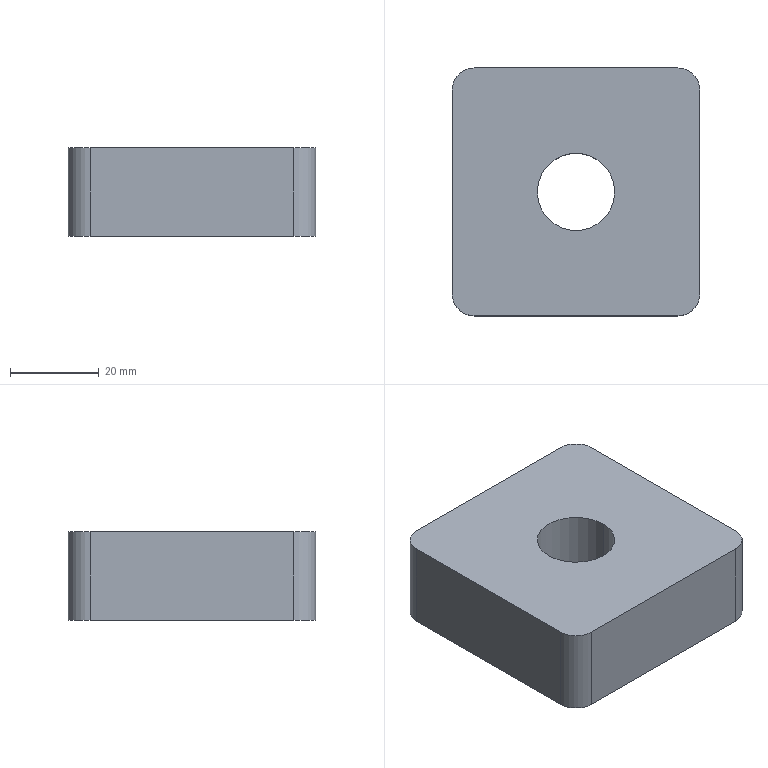Part | SolidWorks | features BaseBody 1 | 1 solid | 12 faces | box 56 x 56 x 20 mm | volume 57480 mm3 | cylinder 6 | plane 6 | commonest cylinder face diameters 10 x4 17.5 x2
STEP:
#1=CARTESIAN_POINT('',(678.75,22.,-1560.));
#2=VERTEX_POINT('',#1);
#3=CARTESIAN_POINT('',(661.25,22.,-1560.));
#4=VERTEX_POINT('',#3);
#5=CARTESIAN_POINT('',(670.,22.,-1560.));
#6=DIRECTION('',(0.,0.,-1.));
#7=DIRECTION('',(-1.,0.,0.));
#8=AXIS2_PLACEMENT_3D('',#5,#6,#7);
#9=CIRCLE('',#8,8.75);
#10=EDGE_CURVE('',#2,#4,#9,.T.);
#11=ORIENTED_EDGE('',*,*,#10,.F.);
#12=CARTESIAN_POINT('',(678.75,22.,-1580.));
#13=VERTEX_POINT('',#12);
#14=CARTESIAN_POINT('',(678.75,22.,-1580.));
#15=DIRECTION('',(0.,0.,-1.));
#16=VECTOR('',#15,1000.);
#17=LINE('',#14,#16);
#18=EDGE_CURVE('',#2,#13,#17,.T.);
#19=ORIENTED_EDGE('',*,*,#18,.T.);
#20=CARTESIAN_POINT('',(661.25,22.,-1580.));
#21=VERTEX_POINT('',#20);
#22=CARTESIAN_POINT('',(670.,22.,-1580.));
#23=DIRECTION('',(0.,0.,-1.));
#24=DIRECTION('',(-1.,0.,0.));
#25=AXIS2_PLACEMENT_3D('',#22,#23,#24);
#26=CIRCLE('',#25,8.75);
#27=EDGE_CURVE('',#13,#21,#26,.T.);
#28=ORIENTED_EDGE('',*,*,#27,.T.);
#29=CARTESIAN_POINT('',(661.25,22.,-1580.));
#30=DIRECTION('',(0.,0.,-1.));
#31=VECTOR('',#30,1000.);
#32=LINE('',#29,#31);
#33=EDGE_CURVE('',#4,#21,#32,.T.);
#34=ORIENTED_EDGE('',*,*,#33,.F.);
#35=EDGE_LOOP('',(#11,#19,#28,#34));
#36=FACE_OUTER_BOUND('',#35,.T.);
#37=CARTESIAN_POINT('',(670.,22.,-1580.));
#38=DIRECTION('',(0.,0.,-1.));
#39=DIRECTION('',(-1.,0.,0.));
#40=AXIS2_PLACEMENT_3D('',#37,#38,#39);
#41=CYLINDRICAL_SURFACE('',#40,8.75);
#42=ADVANCED_FACE('',(#36),#41,.F.);
#43=CARTESIAN_POINT('',(670.,22.,-1580.));
#44=DIRECTION('',(0.,0.,-1.));
#45=DIRECTION('',(-1.,0.,0.));
#46=AXIS2_PLACEMENT_3D('',#43,#44,#45);
#47=CIRCLE('',#46,8.75);
#48=EDGE_CURVE('',#21,#13,#47,.T.);
#49=ORIENTED_EDGE('',*,*,#48,.F.);
#50=ORIENTED_EDGE('',*,*,#27,.F.);
#51=EDGE_LOOP('',(#49,#50));
#52=FACE_BOUND('',#51,.T.);
#53=CARTESIAN_POINT('',(698.,-1.,-1580.));
#54=VERTEX_POINT('',#53);
#55=CARTESIAN_POINT('',(698.,45.,-1580.));
#56=VERTEX_POINT('',#55);
#57=CARTESIAN_POINT('',(698.,45.,-1580.));
#58=DIRECTION('',(0.,1.,0.));
#59=VECTOR('',#58,1000.);
#60=LINE('',#57,#59);
#61=EDGE_CURVE('',#54,#56,#60,.T.);
#62=ORIENTED_EDGE('',*,*,#61,.F.);
#63=CARTESIAN_POINT('',(693.,-6.,-1580.));
#64=VERTEX_POINT('',#63);
#65=CARTESIAN_POINT('',(693.,-1.,-1580.));
#66=DIRECTION('',(0.,0.,1.));
#67=DIRECTION('',(1.,0.,0.));
#68=AXIS2_PLACEMENT_3D('',#65,#66,#67);
#69=CIRCLE('',#68,5.);
#70=EDGE_CURVE('',#64,#54,#69,.T.);
#71=ORIENTED_EDGE('',*,*,#70,.F.);
#72=CARTESIAN_POINT('',(647.,-6.,-1580.));
#73=VERTEX_POINT('',#72);
#74=CARTESIAN_POINT('',(693.,-6.,-1580.));
#75=DIRECTION('',(1.,0.,0.));
#76=VECTOR('',#75,1000.);
#77=LINE('',#74,#76);
#78=EDGE_CURVE('',#73,#64,#77,.T.);
#79=ORIENTED_EDGE('',*,*,#78,.F.);
#80=CARTESIAN_POINT('',(642.,-1.,-1580.));
#81=VERTEX_POINT('',#80);
#82=CARTESIAN_POINT('',(647.,-1.,-1580.));
#83=DIRECTION('',(0.,0.,1.));
#84=DIRECTION('',(1.,0.,0.));
#85=AXIS2_PLACEMENT_3D('',#82,#83,#84);
#86=CIRCLE('',#85,5.);
#87=EDGE_CURVE('',#81,#73,#86,.T.);
#88=ORIENTED_EDGE('',*,*,#87,.F.);
#89=CARTESIAN_POINT('',(642.,45.,-1580.));
#90=VERTEX_POINT('',#89);
#91=CARTESIAN_POINT('',(642.,45.,-1580.));
#92=DIRECTION('',(0.,-1.,0.));
#93=VECTOR('',#92,1000.);
#94=LINE('',#91,#93);
#95=EDGE_CURVE('',#90,#81,#94,.T.);
#96=ORIENTED_EDGE('',*,*,#95,.F.);
#97=CARTESIAN_POINT('',(647.,50.,-1580.));
#98=VERTEX_POINT('',#97);
#99=CARTESIAN_POINT('',(647.,45.,-1580.));
#100=DIRECTION('',(0.,0.,1.));
#101=DIRECTION('',(1.,0.,0.));
#102=AXIS2_PLACEMENT_3D('',#99,#100,#101);
#103=CIRCLE('',#102,5.);
#104=EDGE_CURVE('',#98,#90,#103,.T.);
#105=ORIENTED_EDGE('',*,*,#104,.F.);
#106=CARTESIAN_POINT('',(693.,50.,-1580.));
#107=VERTEX_POINT('',#106);
#108=CARTESIAN_POINT('',(693.,50.,-1580.));
#109=DIRECTION('',(-1.,0.,0.));
#110=VECTOR('',#109,1000.);
#111=LINE('',#108,#110);
#112=EDGE_CURVE('',#107,#98,#111,.T.);
#113=ORIENTED_EDGE('',*,*,#112,.F.);
#114=CARTESIAN_POINT('',(693.,45.,-1580.));
#115=DIRECTION('',(0.,0.,1.));
#116=DIRECTION('',(1.,0.,0.));
#117=AXIS2_PLACEMENT_3D('',#114,#115,#116);
#118=CIRCLE('',#117,5.);
#119=EDGE_CURVE('',#56,#107,#118,.T.);
#120=ORIENTED_EDGE('',*,*,#119,.F.);
#121=EDGE_LOOP('',(#62,#71,#79,#88,#96,#105,#113,#120));
#122=FACE_OUTER_BOUND('',#121,.T.);
#123=CARTESIAN_POINT('',(693.,45.,-1580.));
#124=DIRECTION('',(0.,0.,1.));
#125=DIRECTION('',(1.,0.,0.));
#126=AXIS2_PLACEMENT_3D('',#123,#124,#125);
#127=PLANE('',#126);
#128=ADVANCED_FACE('',(#52,#122),#127,.F.);
#129=ORIENTED_EDGE('',*,*,#18,.F.);
#130=CARTESIAN_POINT('',(670.,22.,-1560.));
#131=DIRECTION('',(0.,0.,-1.));
#132=DIRECTION('',(-1.,0.,0.));
#133=AXIS2_PLACEMENT_3D('',#130,#131,#132);
#134=CIRCLE('',#133,8.75);
#135=EDGE_CURVE('',#4,#2,#134,.T.);
#136=ORIENTED_EDGE('',*,*,#135,.F.);
#137=ORIENTED_EDGE('',*,*,#33,.T.);
#138=ORIENTED_EDGE('',*,*,#48,.T.);
#139=EDGE_LOOP('',(#129,#136,#137,#138));
#140=FACE_OUTER_BOUND('',#139,.T.);
#141=CARTESIAN_POINT('',(670.,22.,-1580.));
#142=DIRECTION('',(0.,0.,-1.));
#143=DIRECTION('',(-1.,0.,0.));
#144=AXIS2_PLACEMENT_3D('',#141,#142,#143);
#145=CYLINDRICAL_SURFACE('',#144,8.75);
#146=ADVANCED_FACE('',(#140),#145,.F.);
#147=CARTESIAN_POINT('',(693.,50.,-1560.));
#148=VERTEX_POINT('',#147);
#149=CARTESIAN_POINT('',(693.,50.,-1580.));
#150=DIRECTION('',(0.,0.,1.));
#151=VECTOR('',#150,1000.);
#152=LINE('',#149,#151);
#153=EDGE_CURVE('',#107,#148,#152,.T.);
#154=ORIENTED_EDGE('',*,*,#153,.T.);
#155=CARTESIAN_POINT('',(698.,45.,-1560.));
#156=VERTEX_POINT('',#155);
#157=CARTESIAN_POINT('',(693.,45.,-1560.));
#158=DIRECTION('',(0.,0.,-1.));
#159=DIRECTION('',(1.,0.,0.));
#160=AXIS2_PLACEMENT_3D('',#157,#158,#159);
#161=CIRCLE('',#160,5.);
#162=EDGE_CURVE('',#148,#156,#161,.T.);
#163=ORIENTED_EDGE('',*,*,#162,.T.);
#164=CARTESIAN_POINT('',(698.,45.,-1580.));
#165=DIRECTION('',(0.,0.,-1.));
#166=VECTOR('',#165,1000.);
#167=LINE('',#164,#166);
#168=EDGE_CURVE('',#156,#56,#167,.T.);
#169=ORIENTED_EDGE('',*,*,#168,.T.);
#170=ORIENTED_EDGE('',*,*,#119,.T.);
#171=EDGE_LOOP('',(#154,#163,#169,#170));
#172=FACE_OUTER_BOUND('',#171,.T.);
#173=CARTESIAN_POINT('',(693.,45.,-1580.));
#174=DIRECTION('',(0.,0.,1.));
#175=DIRECTION('',(1.,0.,0.));
#176=AXIS2_PLACEMENT_3D('',#173,#174,#175);
#177=CYLINDRICAL_SURFACE('',#176,5.);
#178=ADVANCED_FACE('',(#172),#177,.T.);
#179=ORIENTED_EDGE('',*,*,#61,.T.);
#180=ORIENTED_EDGE('',*,*,#168,.F.);
#181=CARTESIAN_POINT('',(698.,-1.,-1560.));
#182=VERTEX_POINT('',#181);
#183=CARTESIAN_POINT('',(698.,50.,-1560.));
#184=DIRECTION('',(0.,1.,0.));
#185=VECTOR('',#184,1000.);
#186=LINE('',#183,#185);
#187=EDGE_CURVE('',#182,#156,#186,.T.);
#188=ORIENTED_EDGE('',*,*,#187,.F.);
#189=CARTESIAN_POINT('',(698.,-1.,-1580.));
#190=DIRECTION('',(0.,0.,1.));
#191=VECTOR('',#190,1000.);
#192=LINE('',#189,#191);
#193=EDGE_CURVE('',#54,#182,#192,.T.);
#194=ORIENTED_EDGE('',*,*,#193,.F.);
#195=EDGE_LOOP('',(#179,#180,#188,#194));
#196=FACE_OUTER_BOUND('',#195,.T.);
#197=CARTESIAN_POINT('',(698.,50.,-1580.));
#198=DIRECTION('',(-1.,0.,0.));
#199=DIRECTION('',(0.,0.,1.));
#200=AXIS2_PLACEMENT_3D('',#197,#198,#199);
#201=PLANE('',#200);
#202=ADVANCED_FACE('',(#196),#201,.F.);
#203=ORIENTED_EDGE('',*,*,#193,.T.);
#204=CARTESIAN_POINT('',(693.,-6.,-1560.));
#205=VERTEX_POINT('',#204);
#206=CARTESIAN_POINT('',(693.,-1.,-1560.));
#207=DIRECTION('',(0.,0.,-1.));
#208=DIRECTION('',(1.,0.,0.));
#209=AXIS2_PLACEMENT_3D('',#206,#207,#208);
#210=CIRCLE('',#209,5.);
#211=EDGE_CURVE('',#182,#205,#210,.T.);
#212=ORIENTED_EDGE('',*,*,#211,.T.);
#213=CARTESIAN_POINT('',(693.,-6.,-1580.));
#214=DIRECTION('',(0.,0.,-1.));
#215=VECTOR('',#214,1000.);
#216=LINE('',#213,#215);
#217=EDGE_CURVE('',#205,#64,#216,.T.);
#218=ORIENTED_EDGE('',*,*,#217,.T.);
#219=ORIENTED_EDGE('',*,*,#70,.T.);
#220=EDGE_LOOP('',(#203,#212,#218,#219));
#221=FACE_OUTER_BOUND('',#220,.T.);
#222=CARTESIAN_POINT('',(693.,-1.,-1580.));
#223=DIRECTION('',(0.,0.,1.));
#224=DIRECTION('',(1.,0.,0.));
#225=AXIS2_PLACEMENT_3D('',#222,#223,#224);
#226=CYLINDRICAL_SURFACE('',#225,5.);
#227=ADVANCED_FACE('',(#221),#226,.T.);
#228=ORIENTED_EDGE('',*,*,#78,.T.);
#229=ORIENTED_EDGE('',*,*,#217,.F.);
#230=CARTESIAN_POINT('',(647.,-6.,-1560.));
#231=VERTEX_POINT('',#230);
#232=CARTESIAN_POINT('',(698.,-6.,-1560.));
#233=DIRECTION('',(1.,0.,0.));
#234=VECTOR('',#233,1000.);
#235=LINE('',#232,#234);
#236=EDGE_CURVE('',#231,#205,#235,.T.);
#237=ORIENTED_EDGE('',*,*,#236,.F.);
#238=CARTESIAN_POINT('',(647.,-6.,-1580.));
#239=DIRECTION('',(0.,0.,1.));
#240=VECTOR('',#239,1000.);
#241=LINE('',#238,#240);
#242=EDGE_CURVE('',#73,#231,#241,.T.);
#243=ORIENTED_EDGE('',*,*,#242,.F.);
#244=EDGE_LOOP('',(#228,#229,#237,#243));
#245=FACE_OUTER_BOUND('',#244,.T.);
#246=CARTESIAN_POINT('',(698.,-6.,-1580.));
#247=DIRECTION('',(0.,1.,0.));
#248=DIRECTION('',(0.,0.,1.));
#249=AXIS2_PLACEMENT_3D('',#246,#247,#248);
#250=PLANE('',#249);
#251=ADVANCED_FACE('',(#245),#250,.F.);
#252=ORIENTED_EDGE('',*,*,#242,.T.);
#253=CARTESIAN_POINT('',(642.,-1.,-1560.));
#254=VERTEX_POINT('',#253);
#255=CARTESIAN_POINT('',(647.,-1.,-1560.));
#256=DIRECTION('',(0.,0.,-1.));
#257=DIRECTION('',(1.,0.,0.));
#258=AXIS2_PLACEMENT_3D('',#255,#256,#257);
#259=CIRCLE('',#258,5.);
#260=EDGE_CURVE('',#231,#254,#259,.T.);
#261=ORIENTED_EDGE('',*,*,#260,.T.);
#262=CARTESIAN_POINT('',(642.,-1.,-1580.));
#263=DIRECTION('',(0.,0.,-1.));
#264=VECTOR('',#263,1000.);
#265=LINE('',#262,#264);
#266=EDGE_CURVE('',#254,#81,#265,.T.);
#267=ORIENTED_EDGE('',*,*,#266,.T.);
#268=ORIENTED_EDGE('',*,*,#87,.T.);
#269=EDGE_LOOP('',(#252,#261,#267,#268));
#270=FACE_OUTER_BOUND('',#269,.T.);
#271=CARTESIAN_POINT('',(647.,-1.,-1580.));
#272=DIRECTION('',(0.,0.,1.));
#273=DIRECTION('',(1.,0.,0.));
#274=AXIS2_PLACEMENT_3D('',#271,#272,#273);
#275=CYLINDRICAL_SURFACE('',#274,5.);
#276=ADVANCED_FACE('',(#270),#275,.T.);
#277=ORIENTED_EDGE('',*,*,#95,.T.);
#278=ORIENTED_EDGE('',*,*,#266,.F.);
#279=CARTESIAN_POINT('',(642.,45.,-1560.));
#280=VERTEX_POINT('',#279);
#281=CARTESIAN_POINT('',(642.,-6.,-1560.));
#282=DIRECTION('',(0.,-1.,0.));
#283=VECTOR('',#282,1000.);
#284=LINE('',#281,#283);
#285=EDGE_CURVE('',#280,#254,#284,.T.);
#286=ORIENTED_EDGE('',*,*,#285,.F.);
#287=CARTESIAN_POINT('',(642.,45.,-1580.));
#288=DIRECTION('',(0.,0.,1.));
#289=VECTOR('',#288,1000.);
#290=LINE('',#287,#289);
#291=EDGE_CURVE('',#90,#280,#290,.T.);
#292=ORIENTED_EDGE('',*,*,#291,.F.);
#293=EDGE_LOOP('',(#277,#278,#286,#292));
#294=FACE_OUTER_BOUND('',#293,.T.);
#295=CARTESIAN_POINT('',(642.,-6.,-1580.));
#296=DIRECTION('',(1.,0.,0.));
#297=DIRECTION('',(0.,0.,-1.));
#298=AXIS2_PLACEMENT_3D('',#295,#296,#297);
#299=PLANE('',#298);
#300=ADVANCED_FACE('',(#294),#299,.F.);
#301=ORIENTED_EDGE('',*,*,#291,.T.);
#302=CARTESIAN_POINT('',(647.,50.,-1560.));
#303=VERTEX_POINT('',#302);
#304=CARTESIAN_POINT('',(647.,45.,-1560.));
#305=DIRECTION('',(0.,0.,-1.));
#306=DIRECTION('',(1.,0.,0.));
#307=AXIS2_PLACEMENT_3D('',#304,#305,#306);
#308=CIRCLE('',#307,5.);
#309=EDGE_CURVE('',#280,#303,#308,.T.);
#310=ORIENTED_EDGE('',*,*,#309,.T.);
#311=CARTESIAN_POINT('',(647.,50.,-1580.));
#312=DIRECTION('',(0.,0.,-1.));
#313=VECTOR('',#312,1000.);
#314=LINE('',#311,#313);
#315=EDGE_CURVE('',#303,#98,#314,.T.);
#316=ORIENTED_EDGE('',*,*,#315,.T.);
#317=ORIENTED_EDGE('',*,*,#104,.T.);
#318=EDGE_LOOP('',(#301,#310,#316,#317));
#319=FACE_OUTER_BOUND('',#318,.T.);
#320=CARTESIAN_POINT('',(647.,45.,-1580.));
#321=DIRECTION('',(0.,0.,1.));
#322=DIRECTION('',(1.,0.,0.));
#323=AXIS2_PLACEMENT_3D('',#320,#321,#322);
#324=CYLINDRICAL_SURFACE('',#323,5.);
#325=ADVANCED_FACE('',(#319),#324,.T.);
#326=ORIENTED_EDGE('',*,*,#112,.T.);
#327=ORIENTED_EDGE('',*,*,#315,.F.);
#328=CARTESIAN_POINT('',(642.,50.,-1560.));
#329=DIRECTION('',(-1.,0.,0.));
#330=VECTOR('',#329,1000.);
#331=LINE('',#328,#330);
#332=EDGE_CURVE('',#148,#303,#331,.T.);
#333=ORIENTED_EDGE('',*,*,#332,.F.);
#334=ORIENTED_EDGE('',*,*,#153,.F.);
#335=EDGE_LOOP('',(#326,#327,#333,#334));
#336=FACE_OUTER_BOUND('',#335,.T.);
#337=CARTESIAN_POINT('',(642.,50.,-1580.));
#338=DIRECTION('',(0.,-1.,0.));
#339=DIRECTION('',(0.,0.,-1.));
#340=AXIS2_PLACEMENT_3D('',#337,#338,#339);
#341=PLANE('',#340);
#342=ADVANCED_FACE('',(#336),#341,.F.);
#343=ORIENTED_EDGE('',*,*,#135,.T.);
#344=ORIENTED_EDGE('',*,*,#10,.T.);
#345=EDGE_LOOP('',(#343,#344));
#346=FACE_BOUND('',#345,.T.);
#347=ORIENTED_EDGE('',*,*,#162,.F.);
#348=ORIENTED_EDGE('',*,*,#332,.T.);
#349=ORIENTED_EDGE('',*,*,#309,.F.);
#350=ORIENTED_EDGE('',*,*,#285,.T.);
#351=ORIENTED_EDGE('',*,*,#260,.F.);
#352=ORIENTED_EDGE('',*,*,#236,.T.);
#353=ORIENTED_EDGE('',*,*,#211,.F.);
#354=ORIENTED_EDGE('',*,*,#187,.T.);
#355=EDGE_LOOP('',(#347,#348,#349,#350,#351,#352,#353,#354));
#356=FACE_OUTER_BOUND('',#355,.T.);
#357=CARTESIAN_POINT('',(693.,45.,-1560.));
#358=DIRECTION('',(0.,0.,1.));
#359=DIRECTION('',(1.,0.,0.));
#360=AXIS2_PLACEMENT_3D('',#357,#358,#359);
#361=PLANE('',#360);
#362=ADVANCED_FACE('',(#346,#356),#361,.T.);
#363=CLOSED_SHELL('',(#42,#128,#146,#178,#202,#227,#251,#276,#300,#325,#342,#362));
#364=MANIFOLD_SOLID_BREP('',#363);
#365=CARTESIAN_POINT('',(0.,0.,0.));
#366=DIRECTION('',(0.,0.,1.));
#367=DIRECTION('',(1.,0.,0.));
#368=AXIS2_PLACEMENT_3D('',#365,#366,#367);
#369=(LENGTH_UNIT()NAMED_UNIT(*)SI_UNIT(.MILLI.,.METRE.));
#370=UNCERTAINTY_MEASURE_WITH_UNIT(LENGTH_MEASURE(0.00001),#369,'','');
#371=(NAMED_UNIT(*)PLANE_ANGLE_UNIT()SI_UNIT($,.RADIAN.));
#372=(NAMED_UNIT(*)SI_UNIT($,.STERADIAN.)SOLID_ANGLE_UNIT());
#373=(GEOMETRIC_REPRESENTATION_CONTEXT(3)GLOBAL_UNCERTAINTY_ASSIGNED_CONTEXT((#370))GLOBAL_UNIT_ASSIGNED_CONTEXT((#369,#371,#372))REPRESENTATION_CONTEXT('',''));
#374=ADVANCED_BREP_SHAPE_REPRESENTATION('',(#364,#368),#373);